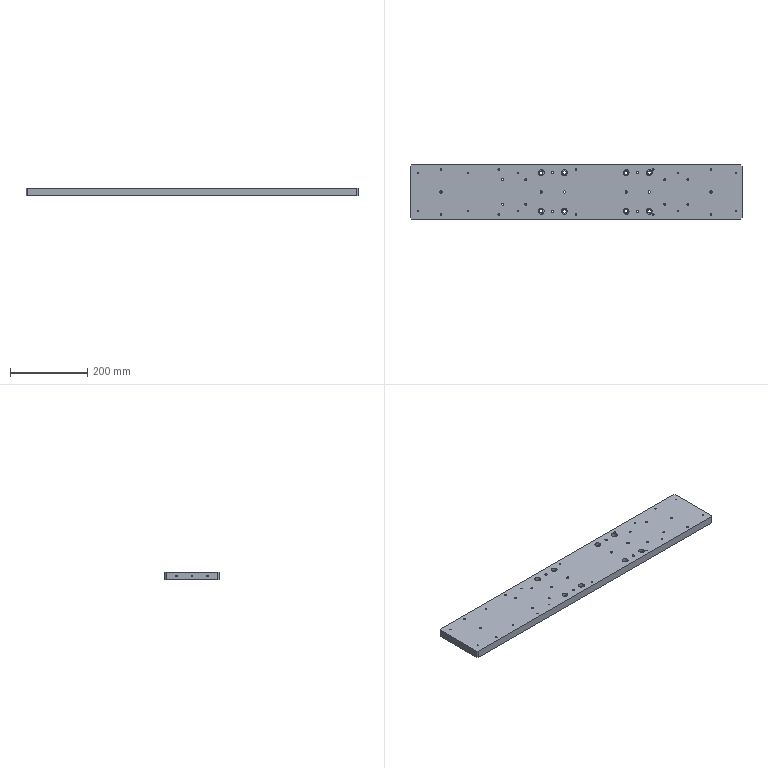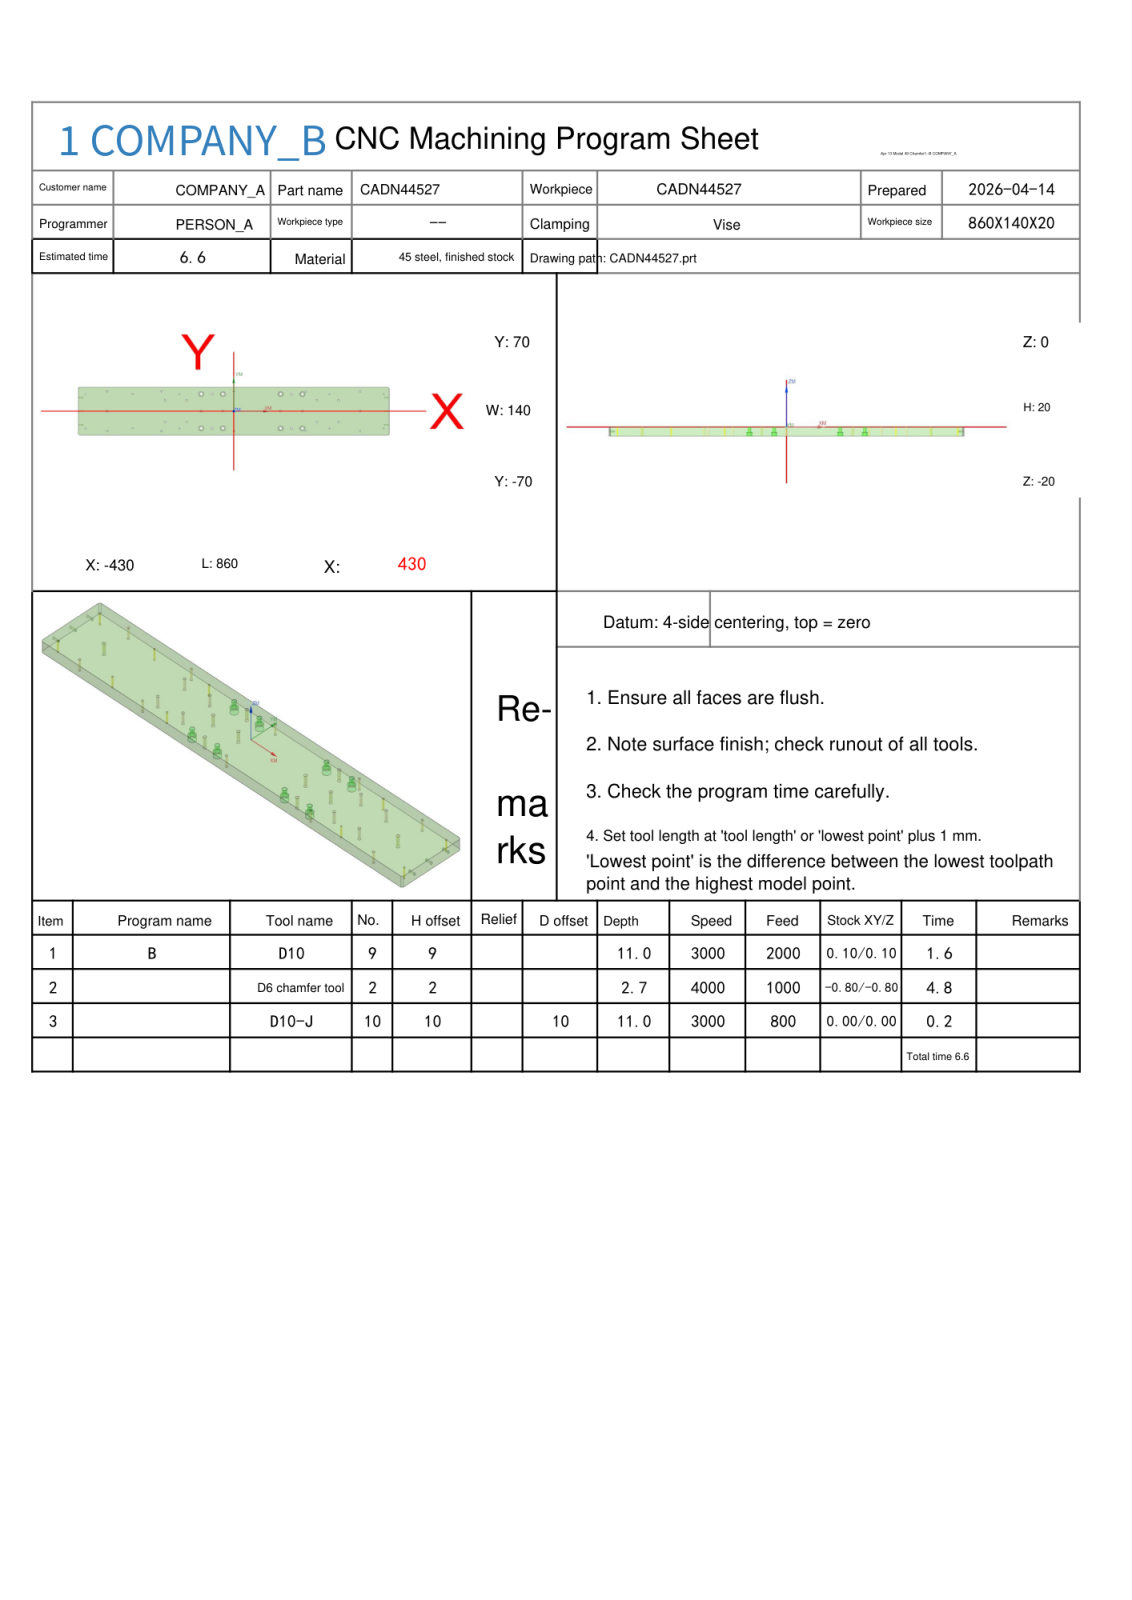NC program | NX | posted by the shop | part box 860 x 140 x 20 mm
Whole program:
%
O0001
(Machine time: 7.09 MIN)
(===Total Tool:3===)
(T9=D10     D=10.  R=0.   D-  H09 Z=-11.  )
(T2=D6 chamfer tool   D=6.   R=0.   D-  H02 Z=-2.7  )
(T10=D10-J  D=10.  R=0.   D10 H10 Z=-11.  )
G80 G90 G17 G49 G40
G91 G28 Z0
M01
N1 T09 M06
(D10  D=10. R=0. H=09 ce=0.10 di=0.10)
G00 G90 G54 X-424.112 Y-80.1 M03 S3000
G43 H09 Z20.
M08
Z-.344
G01 X-430.606 Y-73.606 F2000.
X-433.606 Y-70.606
X-440.1 Y-64.112
G00 Z-.688
G01 X-433.606 Y-70.606
X-430.606 Y-73.606
X-424.112 Y-80.1
G00 Z-1.031
G01 X-430.606 Y-73.606
X-433.606 Y-70.606
X-440.1 Y-64.112
G00 Z-1.375
G01 X-433.606 Y-70.606
X-430.606 Y-73.606
X-424.112 Y-80.1
G00 Z-1.719
G01 X-430.606 Y-73.606
X-433.606 Y-70.606
X-440.1 Y-64.112
G00 Z-2.063
G01 X-433.606 Y-70.606
X-430.606 Y-73.606
X-424.112 Y-80.1
G00 Z-2.406
G01 X-430.606 Y-73.606
X-433.606 Y-70.606
X-440.1 Y-64.112
G00 Z-2.75
G01 X-433.606 Y-70.606
X-430.606 Y-73.606
X-424.112 Y-80.1
G00 Z-3.094
G01 X-430.606 Y-73.606
X-433.606 Y-70.606
X-440.1 Y-64.112
G00 Z-3.438
G01 X-433.606 Y-70.606
X-430.606 Y-73.606
X-424.112 Y-80.1
G00 Z-3.781
G01 X-430.606 Y-73.606
X-433.606 Y-70.606
X-440.1 Y-64.112
G00 Z-4.125
G01 X-433.606 Y-70.606
X-430.606 Y-73.606
X-424.112 Y-80.1
G00 Z-4.469
G01 X-430.606 Y-73.606
X-433.606 Y-70.606
X-440.1 Y-64.112
G00 Z-4.813
G01 X-433.606 Y-70.606
X-430.606 Y-73.606
X-424.112 Y-80.1
G00 Z-5.156
G01 X-430.606 Y-73.606
X-433.606 Y-70.606
X-440.1 Y-64.112
G00 Z-5.5
G01 X-433.606 Y-70.606
X-430.606 Y-73.606
X-424.112 Y-80.1
G00 Z-5.844
G01 X-430.606 Y-73.606
X-433.606 Y-70.606
X-440.1 Y-64.112
G00 Z-6.188
G01 X-433.606 Y-70.606
X-430.606 Y-73.606
X-424.112 Y-80.1
G00 Z-6.531
G01 X-430.606 Y-73.606
X-433.606 Y-70.606
X-440.1 Y-64.112
G00 Z-6.875
G01 X-433.606 Y-70.606
X-430.606 Y-73.606
X-424.112 Y-80.1
G00 Z-7.219
G01 X-430.606 Y-73.606
X-433.606 Y-70.606
X-440.1 Y-64.112
G00 Z-7.563
G01 X-433.606 Y-70.606
X-430.606 Y-73.606
X-424.112 Y-80.1
G00 Z-7.906
G01 X-430.606 Y-73.606
X-433.606 Y-70.606
X-440.1 Y-64.112
G00 Z-8.25
G01 X-433.606 Y-70.606
X-430.606 Y-73.606
X-424.112 Y-80.1
G00 Z-8.594
G01 X-430.606 Y-73.606
X-433.606 Y-70.606
X-440.1 Y-64.112
G00 Z-8.938
G01 X-433.606 Y-70.606
X-430.606 Y-73.606
X-424.112 Y-80.1
G00 Z-9.281
G01 X-430.606 Y-73.606
X-433.606 Y-70.606
X-440.1 Y-64.112
G00 Z-9.625
G01 X-433.606 Y-70.606
X-430.606 Y-73.606
X-424.112 Y-80.1
G00 Z-9.969
G01 X-430.606 Y-73.606
X-433.606 Y-70.606
X-440.1 Y-64.112
G00 Z-10.313
G01 X-433.606 Y-70.606
X-430.606 Y-73.606
X-424.112 Y-80.1
G00 Z-10.656
G01 X-430.606 Y-73.606
X-433.606 Y-70.606
X-440.1 Y-64.112
G00 Z-11.
G01 X-433.606 Y-70.606
X-430.606 Y-73.606
X-424.112 Y-80.1
G00 Z20.
X-440.1 Y64.112
Z-.344
G01 X-433.606 Y70.606
X-430.606 Y73.606
X-424.112 Y80.1
G00 Z-.688
G01 X-430.606 Y73.606
X-433.606 Y70.606
X-440.1 Y64.112
G00 Z-1.031
G01 X-433.606 Y70.606
X-430.606 Y73.606
X-424.112 Y80.1
G00 Z-1.375
G01 X-430.606 Y73.606
X-433.606 Y70.606
X-440.1 Y64.112
G00 Z-1.719
G01 X-433.606 Y70.606
X-430.606 Y73.606
X-424.112 Y80.1
G00 Z-2.063
G01 X-430.606 Y73.606
X-433.606 Y70.606
X-440.1 Y64.112
G00 Z-2.406
G01 X-433.606 Y70.606
X-430.606 Y73.606
X-424.112 Y80.1
G00 Z-2.75
G01 X-430.606 Y73.606
X-433.606 Y70.606
X-440.1 Y64.112
G00 Z-3.094
G01 X-433.606 Y70.606
X-430.606 Y73.606
X-424.112 Y80.1
G00 Z-3.438
G01 X-430.606 Y73.606
X-433.606 Y70.606
X-440.1 Y64.112
G00 Z-3.781
G01 X-433.606 Y70.606
X-430.606 Y73.606
X-424.112 Y80.1
G00 Z-4.125
G01 X-430.606 Y73.606
X-433.606 Y70.606
X-440.1 Y64.112
G00 Z-4.469
G01 X-433.606 Y70.606
X-430.606 Y73.606
X-424.112 Y80.1
G00 Z-4.813
G01 X-430.606 Y73.606
X-433.606 Y70.606
X-440.1 Y64.112
G00 Z-5.156
G01 X-433.606 Y70.606
X-430.606 Y73.606
X-424.112 Y80.1
G00 Z-5.5
G01 X-430.606 Y73.606
X-433.606 Y70.606
X-440.1 Y64.112
G00 Z-5.844
G01 X-433.606 Y70.606
X-430.606 Y73.606
X-424.112 Y80.1
G00 Z-6.188
G01 X-430.606 Y73.606
X-433.606 Y70.606
X-440.1 Y64.112
G00 Z-6.531
G01 X-433.606 Y70.606
X-430.606 Y73.606
X-424.112 Y80.1
G00 Z-6.875
G01 X-430.606 Y73.606
X-433.606 Y70.606
X-440.1 Y64.112
G00 Z-7.219
G01 X-433.606 Y70.606
X-430.606 Y73.606
X-424.112 Y80.1
G00 Z-7.563
G01 X-430.606 Y73.606
X-433.606 Y70.606
X-440.1 Y64.112
G00 Z-7.906
G01 X-433.606 Y70.606
X-430.606 Y73.606
X-424.112 Y80.1
G00 Z-8.25
G01 X-430.606 Y73.606
X-433.606 Y70.606
X-440.1 Y64.112
G00 Z-8.594
G01 X-433.606 Y70.606
X-430.606 Y73.606
X-424.112 Y80.1
G00 Z-8.938
G01 X-430.606 Y73.606
X-433.606 Y70.606
X-440.1 Y64.112
G00 Z-9.281
G01 X-433.606 Y70.606
X-430.606 Y73.606
X-424.112 Y80.1
G00 Z-9.625
G01 X-430.606 Y73.606
X-433.606 Y70.606
X-440.1 Y64.112
G00 Z-9.969
G01 X-433.606 Y70.606
X-430.606 Y73.606
X-424.112 Y80.1
G00 Z-10.313
G01 X-430.606 Y73.606
X-433.606 Y70.606
X-440.1 Y64.112
G00 Z-10.656
G01 X-433.606 Y70.606
X-430.606 Y73.606
X-424.112 Y80.1
G00 Z-11.
G01 X-430.606 Y73.606
X-433.606 Y70.606
X-440.1 Y64.112
G00 Z20.
X424.112 Y80.1
Z-.344
G01 X430.606 Y73.606
X433.606 Y70.606
X440.1 Y64.112
G00 Z-.688
G01 X433.606 Y70.606
X430.606 Y73.606
X424.112 Y80.1
G00 Z-1.031
G01 X430.606 Y73.606
X433.606 Y70.606
X440.1 Y64.112
G00 Z-1.375
G01 X433.606 Y70.606
X430.606 Y73.606
X424.112 Y80.1
G00 Z-1.719
G01 X430.606 Y73.606
X433.606 Y70.606
X440.1 Y64.112
G00 Z-2.063
G01 X433.606 Y70.606
X430.606 Y73.606
X424.112 Y80.1
G00 Z-2.406
G01 X430.606 Y73.606
X433.606 Y70.606
X440.1 Y64.112
G00 Z-2.75
G01 X433.606 Y70.606
X430.606 Y73.606
X424.112 Y80.1
G00 Z-3.094
G01 X430.606 Y73.606
X433.606 Y70.606
X440.1 Y64.112
G00 Z-3.438
G01 X433.606 Y70.606
X430.606 Y73.606
X424.112 Y80.1
G00 Z-3.781
G01 X430.606 Y73.606
X433.606 Y70.606
X440.1 Y64.112
G00 Z-4.125
G01 X433.606 Y70.606
X430.606 Y73.606
X424.112 Y80.1
G00 Z-4.469
G01 X430.606 Y73.606
X433.606 Y70.606
X440.1 Y64.112
G00 Z-4.813
G01 X433.606 Y70.606
X430.606 Y73.606
X424.112 Y80.1
G00 Z-5.156
G01 X430.606 Y73.606
X433.606 Y70.606
X440.1 Y64.112
G00 Z-5.5
G01 X433.606 Y70.606
X430.606 Y73.606
X424.112 Y80.1
G00 Z-5.844
G01 X430.606 Y73.606
X433.606 Y70.606
X440.1 Y64.112
G00 Z-6.188
G01 X433.606 Y70.606
X430.606 Y73.606
X424.112 Y80.1
G00 Z-6.531
G01 X430.606 Y73.606
X433.606 Y70.606
X440.1 Y64.112
G00 Z-6.875
G01 X433.606 Y70.606
X430.606 Y73.606
X424.112 Y80.1
G00 Z-7.219
G01 X430.606 Y73.606
X433.606 Y70.606
X440.1 Y64.112
G00 Z-7.563
G01 X433.606 Y70.606
X430.606 Y73.606
X424.112 Y80.1
G00 Z-7.906
G01 X430.606 Y73.606
X433.606 Y70.606
X440.1 Y64.112
G00 Z-8.25
G01 X433.606 Y70.606
X430.606 Y73.606
X424.112 Y80.1
G00 Z-8.594
G01 X430.606 Y73.606
X433.606 Y70.606
X440.1 Y64.112
G00 Z-8.938
G01 X433.606 Y70.606
X430.606 Y73.606
X424.112 Y80.1
G00 Z-9.281
G01 X430.606 Y73.606
X433.606 Y70.606
X440.1 Y64.112
G00 Z-9.625
G01 X433.606 Y70.606
X430.606 Y73.606
X424.112 Y80.1
G00 Z-9.969
G01 X430.606 Y73.606
X433.606 Y70.606
X440.1 Y64.112
G00 Z-10.313
G01 X433.606 Y70.606
X430.606 Y73.606
X424.112 Y80.1
G00 Z-10.656
G01 X430.606 Y73.606
X433.606 Y70.606
X440.1 Y64.112
G00 Z-11.
G01 X433.606 Y70.606
X430.606 Y73.606
X424.112 Y80.1
G00 Z20.
X440.1 Y-64.112
Z-.344
G01 X433.606 Y-70.606
X430.606 Y-73.606
X424.112 Y-80.1
G00 Z-.688
G01 X430.606 Y-73.606
X433.606 Y-70.606
X440.1 Y-64.112
G00 Z-1.031
G01 X433.606 Y-70.606
X430.606 Y-73.606
X424.112 Y-80.1
G00 Z-1.375
G01 X430.606 Y-73.606
X433.606 Y-70.606
X440.1 Y-64.112
G00 Z-1.719
G01 X433.606 Y-70.606
X430.606 Y-73.606
X424.112 Y-80.1
G00 Z-2.063
G01 X430.606 Y-73.606
X433.606 Y-70.606
X440.1 Y-64.112
G00 Z-2.406
G01 X433.606 Y-70.606
X430.606 Y-73.606
X424.112 Y-80.1
G00 Z-2.75
G01 X430.606 Y-73.606
X433.606 Y-70.606
X440.1 Y-64.112
G00 Z-3.094
G01 X433.606 Y-70.606
X430.606 Y-73.606
X424.112 Y-80.1
G00 Z-3.438
G01 X430.606 Y-73.606
X433.606 Y-70.606
X440.1 Y-64.112
G00 Z-3.781
G01 X433.606 Y-70.606
X430.606 Y-73.606
X424.112 Y-80.1
G00 Z-4.125
G01 X430.606 Y-73.606
X433.606 Y-70.606
X440.1 Y-64.112
G00 Z-4.469
G01 X433.606 Y-70.606
X430.606 Y-73.606
X424.112 Y-80.1
G00 Z-4.813
G01 X430.606 Y-73.606
X433.606 Y-70.606
X440.1 Y-64.112
G00 Z-5.156
G01 X433.606 Y-70.606
X430.606 Y-73.606
X424.112 Y-80.1
G00 Z-5.5
G01 X430.606 Y-73.606
X433.606 Y-70.606
X440.1 Y-64.112
G00 Z-5.844
G01 X433.606 Y-70.606
X430.606 Y-73.606
X424.112 Y-80.1
G00 Z-6.188
G01 X430.606 Y-73.606
X433.606 Y-70.606
X440.1 Y-64.112
G00 Z-6.531
G01 X433.606 Y-70.606
X430.606 Y-73.606
X424.112 Y-80.1
G00 Z-6.875
G01 X430.606 Y-73.606
X433.606 Y-70.606
X440.1 Y-64.112
G00 Z-7.219
G01 X433.606 Y-70.606
X430.606 Y-73.606
X424.112 Y-80.1
G00 Z-7.563
G01 X430.606 Y-73.606
X433.606 Y-70.606
X440.1 Y-64.112
G00 Z-7.906
G01 X433.606 Y-70.606
X430.606 Y-73.606
X424.112 Y-80.1
G00 Z-8.25
G01 X430.606 Y-73.606
X433.606 Y-70.606
X440.1 Y-64.112
G00 Z-8.594
G01 X433.606 Y-70.606
X430.606 Y-73.606
X424.112 Y-80.1
G00 Z-8.938
G01 X430.606 Y-73.606
X433.606 Y-70.606
X440.1 Y-64.112
G00 Z-9.281
G01 X433.606 Y-70.606
X430.606 Y-73.606
X424.112 Y-80.1
G00 Z-9.625
G01 X430.606 Y-73.606
X433.606 Y-70.606
X440.1 Y-64.112
G00 Z-9.969
G01 X433.606 Y-70.606
X430.606 Y-73.606
X424.112 Y-80.1
G00 Z-10.313
G01 X430.606 Y-73.606
X433.606 Y-70.606
X440.1 Y-64.112
G00 Z-10.656
G01 X433.606 Y-70.606
X430.606 Y-73.606
X424.112 Y-80.1
G00 Z-11.
G01 X430.606 Y-73.606
X433.606 Y-70.606
X440.1 Y-64.112
G00 Z20.
G91 G28 Z0.0
M05
M09
G91 G28 Z0.0
M01
N2 T02 M06
(D6 chamfer tool  D=6. R=0. H=02 ce=0.00 di=0.10)
G00 G90 G54 X415. Y50. M03 S2000
G43 H02 Z20.
M08
G98 G81 X415. Y50. Z-2.2 R3. F100.
Y-50.
X265.
Y50.
X-150.
Y-50.
X-280.
Y50.
X-410.
Y-50.
G80
G00 Z20.
G00 G90 X350. Y-58. M03 S2000
Z20.
G98 G81 X350. Y-58. Z-2.7 R3. F100.
Y58.
X200.
Y-58.
X0.0
Y58.
X-200.
Y-58.
X-350.
Y58.
G80
G00 Z20.
G00 G90 X-129.907 Y-32.694 M03 S4000
Z20.
Z-1.1
G01 Z-1.6 F300.
X-129.8 Y-33.5
G03 X-128.3 Y-32. I0.0 J1.5
X-130. Y-30.3 I-1.7 J0.0
X-131.7 Y-32. I0.0 J-1.7
X-130. Y-33.7 I1.7 J0.0
X-128.3 Y-32. I0.0 J1.7
X-129.8 Y-30.5 I-1.5 J0.0
G01 X-129.907 Y-31.306
Z-1.1
G00 Z20.
X-189.907 Y-32.694
Z-1.1
G01 Z-1.6
X-189.8 Y-33.5
G03 X-188.3 Y-32. I0.0 J1.5
X-190. Y-30.3 I-1.7 J0.0
X-191.7 Y-32. I0.0 J-1.7
X-190. Y-33.7 I1.7 J0.0
X-188.3 Y-32. I0.0 J1.7
X-189.8 Y-30.5 I-1.5 J0.0
G01 X-189.907 Y-31.306
Z-1.1
G00 Z20.
Y31.306
Z-1.1
G01 Z-1.6
X-189.8 Y30.5
G03 X-188.3 Y32. I0.0 J1.5
X-190. Y33.7 I-1.7 J0.0
X-191.7 Y32. I0.0 J-1.7
X-190. Y30.3 I1.7 J0.0
X-188.3 Y32. I0.0 J1.7
X-189.8 Y33.5 I-1.5 J0.0
G01 X-189.907 Y32.694
Z-1.1
G00 Z20.
X-129.907 Y31.306
Z-1.1
G01 Z-1.6
X-129.8 Y30.5
G03 X-128.3 Y32. I0.0 J1.5
X-130. Y33.7 I-1.7 J0.0
X-131.7 Y32. I0.0 J-1.7
X-130. Y30.3 I1.7 J0.0
X-128.3 Y32. I0.0 J1.7
X-129.8 Y33.5 I-1.5 J0.0
G01 X-129.907 Y32.694
Z-1.1
G00 Z20.
X230.093 Y31.306
Z-1.1
G01 Z-1.6
X230.2 Y30.5
G03 X231.7 Y32. I0.0 J1.5
X230. Y33.7 I-1.7 J0.0
X228.3 Y32. I0.0 J-1.7
X230. Y30.3 I1.7 J0.0
X231.7 Y32. I0.0 J1.7
X230.2 Y33.5 I-1.5 J0.0
G01 X230.093 Y32.694
Z-1.1
G00 Z20.
X290.093 Y31.306
Z-1.1
G01 Z-1.6
X290.2 Y30.5
G03 X291.7 Y32. I0.0 J1.5
X290. Y33.7 I-1.7 J0.0
X288.3 Y32. I0.0 J-1.7
X290. Y30.3 I1.7 J0.0
X291.7 Y32. I0.0 J1.7
X290.2 Y33.5 I-1.5 J0.0
G01 X290.093 Y32.694
Z-1.1
G00 Z20.
Y-32.694
Z-1.1
G01 Z-1.6
X290.2 Y-33.5
G03 X291.7 Y-32. I0.0 J1.5
X290. Y-30.3 I-1.7 J0.0
X288.3 Y-32. I0.0 J-1.7
X290. Y-33.7 I1.7 J0.0
X291.7 Y-32. I0.0 J1.7
X290.2 Y-30.5 I-1.5 J0.0
G01 X290.093 Y-31.306
Z-1.1
G00 Z20.
X230.093 Y-32.694
Z-1.1
G01 Z-1.6
X230.2 Y-33.5
G03 X231.7 Y-32. I0.0 J1.5
X230. Y-30.3 I-1.7 J0.0
X228.3 Y-32. I0.0 J-1.7
X230. Y-33.7 I1.7 J0.0
X231.7 Y-32. I0.0 J1.7
X230.2 Y-30.5 I-1.5 J0.0
G01 X230.093 Y-31.306
Z-1.1
G00 Z20.
G00 G90 X-349.907 Y-.694 M03 S4000
Z20.
Z-1.1
G01 Z-1.6 F600.
X-349.8 Y-1.5
G03 X-348.3 Y0.0 I0.0 J1.5
X-350. Y1.7 I-1.7 J0.0
X-351.7 Y0.0 I0.0 J-1.7
X-350. Y-1.7 I1.7 J0.0
X-348.3 Y0.0 I0.0 J1.7
X-349.8 Y1.5 I-1.5 J0.0
G01 X-349.907 Y.694
Z-1.1
G00 Z20.
X-90.093
Z-1.1
G01 Z-1.6
X-90.2 Y1.5
G03 X-91.7 Y0.0 I0.0 J-1.5
X-90. Y-1.7 I1.7 J0.0
X-88.3 Y0.0 I0.0 J1.7
X-90. Y1.7 I-1.7 J0.0
X-91.7 Y0.0 I0.0 J-1.7
X-90.2 Y-1.5 I1.5 J0.0
G01 X-90.093 Y-.694
Z-1.1
G00 Z20.
X-60.093 Y50.694
Z-1.1
G01 Z-1.6
X-60.2 Y51.5
G03 X-61.7 Y50. I0.0 J-1.5
X-60. Y48.3 I1.7 J0.0
X-58.3 Y50. I0.0 J1.7
X-60. Y51.7 I-1.7 J0.0
X-61.7 Y50. I0.0 J-1.7
X-60.2 Y48.5 I1.5 J0.0
G01 X-60.093 Y49.306
Z-1.1
G00 Z20.
Y-49.306
Z-1.1
G01 Z-1.6
X-60.2 Y-48.5
G03 X-61.7 Y-50. I0.0 J-1.5
X-60. Y-51.7 I1.7 J0.0
X-58.3 Y-50. I0.0 J1.7
X-60. Y-48.3 I-1.7 J0.0
X-61.7 Y-50. I0.0 J-1.7
X-60.2 Y-51.5 I1.5 J0.0
G01 X-60.093 Y-50.694
Z-1.1
G00 Z20.
X-30.093 Y.694
Z-1.1
G01 Z-1.6
X-30.2 Y1.5
G03 X-31.7 Y0.0 I0.0 J-1.5
X-30. Y-1.7 I1.7 J0.0
X-28.3 Y0.0 I0.0 J1.7
X-30. Y1.7 I-1.7 J0.0
X-31.7 Y0.0 I0.0 J-1.7
X-30.2 Y-1.5 I1.5 J0.0
G01 X-30.093 Y-.694
Z-1.1
G00 Z20.
X129.907 Y.694
Z-1.1
G01 Z-1.6
X129.8 Y1.5
G03 X128.3 Y0.0 I0.0 J-1.5
X130. Y-1.7 I1.7 J0.0
X131.7 Y0.0 I0.0 J1.7
X130. Y1.7 I-1.7 J0.0
X128.3 Y0.0 I0.0 J-1.7
X129.8 Y-1.5 I1.5 J0.0
G01 X129.907 Y-.694
Z-1.1
G00 Z20.
X159.907 Y50.694
Z-1.1
G01 Z-1.6
X159.8 Y51.5
G03 X158.3 Y50. I0.0 J-1.5
X160. Y48.3 I1.7 J0.0
X161.7 Y50. I0.0 J1.7
X160. Y51.7 I-1.7 J0.0
X158.3 Y50. I0.0 J-1.7
X159.8 Y48.5 I1.5 J0.0
G01 X159.907 Y49.306
Z-1.1
G00 Z20.
Y-49.306
Z-1.1
G01 Z-1.6
X159.8 Y-48.5
G03 X158.3 Y-50. I0.0 J-1.5
X160. Y-51.7 I1.7 J0.0
X161.7 Y-50. I0.0 J1.7
X160. Y-48.3 I-1.7 J0.0
X158.3 Y-50. I0.0 J-1.7
X159.8 Y-51.5 I1.5 J0.0
G01 X159.907 Y-50.694
Z-1.1
G00 Z20.
X189.907 Y.694
Z-1.1
G01 Z-1.6
X189.8 Y1.5
G03 X188.3 Y0.0 I0.0 J-1.5
X190. Y-1.7 I1.7 J0.0
X191.7 Y0.0 I0.0 J1.7
X190. Y1.7 I-1.7 J0.0
X188.3 Y0.0 I0.0 J-1.7
X189.8 Y-1.5 I1.5 J0.0
G01 X189.907 Y-.694
Z-1.1
G00 Z20.
X350.093
Z-1.1
G01 Z-1.6
X350.2 Y-1.5
G03 X351.7 Y0.0 I0.0 J1.5
X350. Y1.7 I-1.7 J0.0
X348.3 Y0.0 I0.0 J-1.7
X350. Y-1.7 I1.7 J0.0
X351.7 Y0.0 I0.0 J1.7
X350.2 Y1.5 I-1.5 J0.0
G01 X350.093 Y.694
Z-1.1
G00 Z20.
G00 G90 X130. Y-48.5 M03 S3000
Z20.
Z-1.8
G01 Z-2.3 F600.
X129.
G03 X127.5 Y-50. I0.0 J-1.5
X130. Y-52.5 I2.5 J0.0
X132.5 Y-50. I0.0 J2.5
X130. Y-47.5 I-2.5 J0.0
X127.5 Y-50. I0.0 J-2.5
X129. Y-51.5 I1.5 J0.0
G01 X129.999
Z-1.8
G00 Z20.
X190. Y-48.5
Z-1.8
G01 Z-2.3
X189.
G03 X187.5 Y-50. I0.0 J-1.5
X190. Y-52.5 I2.5 J0.0
X192.5 Y-50. I0.0 J2.5
X190. Y-47.5 I-2.5 J0.0
X187.5 Y-50. I0.0 J-2.5
X189. Y-51.5 I1.5 J0.0
G01 X189.999
Z-1.8
G00 Z20.
X190. Y51.5
Z-1.8
G01 Z-2.3
X189.
G03 X187.5 Y50. I0.0 J-1.5
X190. Y47.5 I2.5 J0.0
X192.5 Y50. I0.0 J2.5
X190. Y52.5 I-2.5 J0.0
X187.5 Y50. I0.0 J-2.5
X189. Y48.5 I1.5 J0.0
G01 X189.999
Z-1.8
G00 Z20.
X130. Y51.5
Z-1.8
G01 Z-2.3
X129.
G03 X127.5 Y50. I0.0 J-1.5
X130. Y47.5 I2.5 J0.0
X132.5 Y50. I0.0 J2.5
X130. Y52.5 I-2.5 J0.0
X127.5 Y50. I0.0 J-2.5
X129. Y48.5 I1.5 J0.0
G01 X129.999
Z-1.8
G00 Z20.
X-30. Y51.5
Z-1.8
G01 Z-2.3
X-31.
G03 X-32.5 Y50. I0.0 J-1.5
X-30. Y47.5 I2.5 J0.0
X-27.5 Y50. I0.0 J2.5
X-30. Y52.5 I-2.5 J0.0
X-32.5 Y50. I0.0 J-2.5
X-31. Y48.5 I1.5 J0.0
G01 X-30.001
Z-1.8
G00 Z20.
X-90. Y51.5
Z-1.8
G01 Z-2.3
X-91.
G03 X-92.5 Y50. I0.0 J-1.5
X-90. Y47.5 I2.5 J0.0
X-87.5 Y50. I0.0 J2.5
X-90. Y52.5 I-2.5 J0.0
X-92.5 Y50. I0.0 J-2.5
X-91. Y48.5 I1.5 J0.0
G01 X-90.001
Z-1.8
G00 Z20.
X-90. Y-48.5
Z-1.8
G01 Z-2.3
X-91.
G03 X-92.5 Y-50. I0.0 J-1.5
X-90. Y-52.5 I2.5 J0.0
X-87.5 Y-50. I0.0 J2.5
X-90. Y-47.5 I-2.5 J0.0
X-92.5 Y-50. I0.0 J-2.5
X-91. Y-51.5 I1.5 J0.0
G01 X-90.001
Z-1.8
G00 Z20.
X-30. Y-48.5
Z-1.8
G01 Z-2.3
X-31.
G03 X-32.5 Y-50. I0.0 J-1.5
X-30. Y-52.5 I2.5 J0.0
X-27.5 Y-50. I0.0 J2.5
X-30. Y-47.5 I-2.5 J0.0
X-32.5 Y-50. I0.0 J-2.5
X-31. Y-51.5 I1.5 J0.0
G01 X-30.
Z-1.8
G00 Z20.
G00 G90 X431.2 Y-57.065 M03 S4000
Z20.
Z2.5
G01 Y-66.876 Z-1.071 F1000.
Y-66.971 Z-1.105
X431.164 Y-67.215 Z-1.195
X431.089 Y-67.451 Z-1.285
X430.975 Y-67.671 Z-1.375
X430.828 Y-67.869 Z-1.465
X430.761 Y-67.936 Z-1.5
X427.936 Y-70.761
G02 X426.876 Y-71.2 I-1.061 J1.061
G01 X-426.876
G02 X-427.936 Y-70.761 I0.0 J1.5
G01 X-430.761 Y-67.936
G02 X-431.2 Y-66.876 I1.061 J1.061
G01 Y66.876
G02 X-430.761 Y67.936 I1.5 J0.0
G01 X-427.936 Y70.761
G02 X-426.876 Y71.2 I1.061 J-1.061
G01 X426.876
G02 X427.936 Y70.761 I0.0 J-1.5
G01 X430.761 Y67.936
G02 X431.2 Y66.876 I-1.061 J-1.061
G01 Y-66.876
G02 X430.761 Y-67.936 I-1.5 J0.0
G01 X430.407 Y-68.29
Z1.
G00 Z20.
G91 G28 Z0.0
M05
M09
G91 G28 Z0.0
M01
N3 T10 M06
(D10-J  D=10. R=0. H=10 ce=0.00 di=0.00)
G00 G90 G54 X430.544 Y75.684 M03 S3000
G43 H10 Z5.007
M08
Z-10.
G01 Z-11. F800.
G41 D10
X430.42 Y75.527
G03 X430.096 Y74.596 I1.176 J-.931
X430.536 Y73.536 I1.5 J0.0
G01 X433.536 Y70.536
G03 X434.596 Y70.096 I1.061 J1.061
X435.527 Y70.42 I0.0 J1.5
G01 G40 X435.684 Y70.544
Z-10.
G00 Z5.007
Y-70.544
Z-10.
G01 Z-11.
G41 D10
X435.527 Y-70.42
G03 X434.596 Y-70.096 I-.931 J-1.176
X433.536 Y-70.536 I0.0 J-1.5
G01 X430.536 Y-73.536
G03 X430.096 Y-74.596 I1.061 J-1.061
X430.42 Y-75.527 I1.5 J0.0
G01 G40 X430.544 Y-75.684
Z-10.
G00 Z5.007
X-430.544
Z-10.
G01 Z-11.
G41 D10
X-430.42 Y-75.527
G03 X-430.096 Y-74.596 I-1.176 J.931
X-430.536 Y-73.536 I-1.5 J0.0
G01 X-433.536 Y-70.536
G03 X-434.596 Y-70.096 I-1.061 J-1.061
X-435.527 Y-70.42 I0.0 J-1.5
G01 G40 X-435.684 Y-70.544
Z-10.
G00 Z5.007
Y70.544
Z-10.
G01 Z-11.
G41 D10
X-435.527 Y70.42
G03 X-434.596 Y70.096 I.931 J1.176
X-433.536 Y70.536 I0.0 J1.5
G01 X-430.536 Y73.536
G03 X-430.096 Y74.596 I-1.061 J1.061
X-430.42 Y75.527 I-1.5 J0.0
G01 G40 X-430.544 Y75.684
Z-10.
G00 Z5.007
M05
M09
G91 G28 Z0.0
G91 G28 Y0.0
M30
%